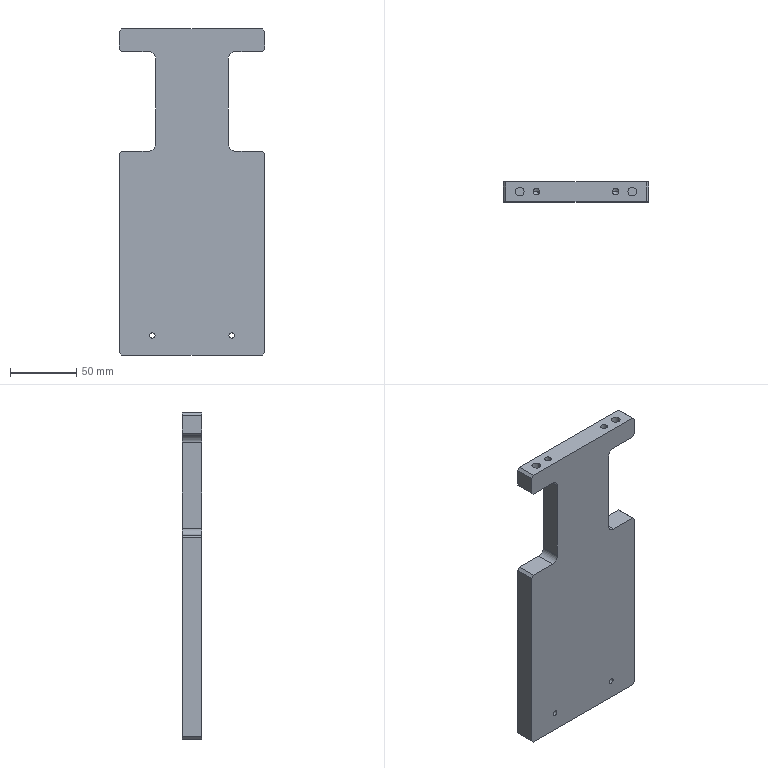Part | STEP file | PN_0012 | 1 solid | 58 faces | box 110 x 15 x 247 mm | volume 337148 mm3 | plane 26 | cylinder 24 | cone 8 | commonest cylinder face diameters 4.2 x8 3 x4 5 x4 6.5 x4 10 x4